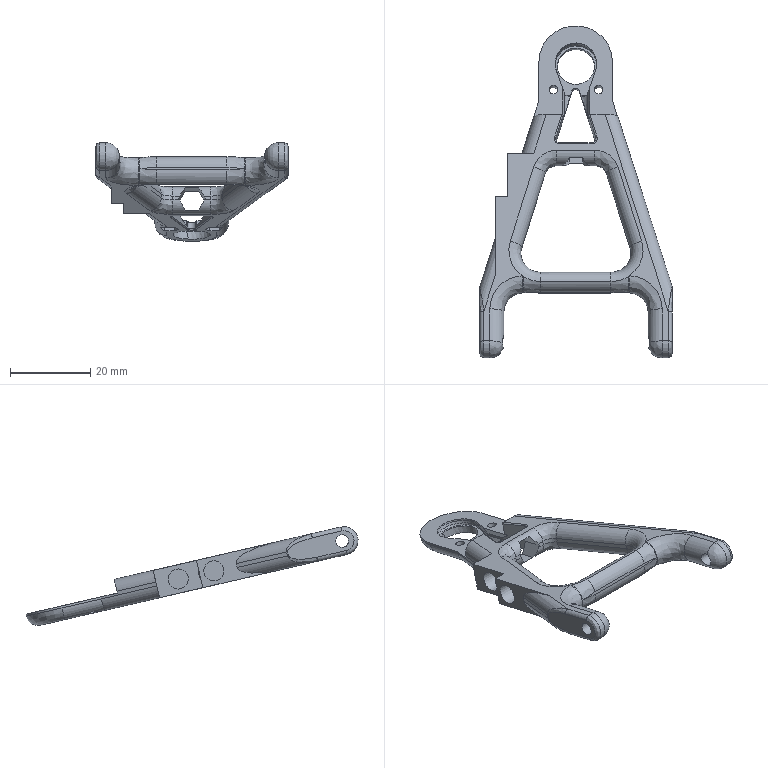Part | STEP file | Wytnij-wyci_gni_cie6_1 | 1 solid | 152 faces | box 48 x 82.899 x 24.651 mm | volume 7377 mm3 | plane 59 | cylinder 56 | spline 37 | commonest cylinder face diameters 6 x20 2 x10 0.6 x6 7 x6 10 x5 2.2 x2